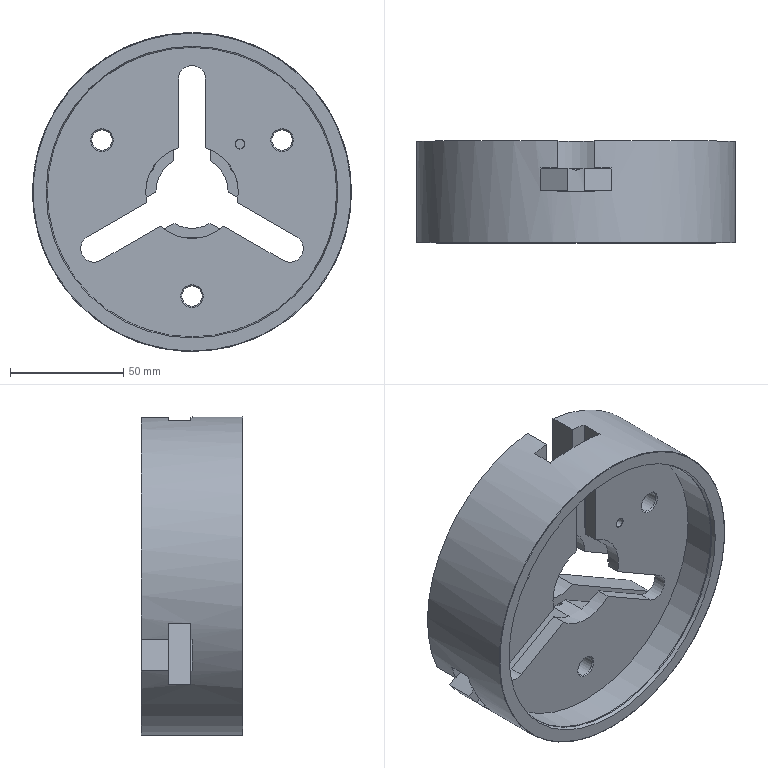CAM job | NX | 3-axis milling, drilling | part box 141 x 45 x 141 mm | stock box 141 x 45 x 141 mm
Tools:
number,name,description,diameter,corner_radius,flute_length,length,flutes
0,D30,Milling Tool-T Cutter,30.0,,9.0,50.0,4
0,D12,Milling Tool-5 Parameters,12.0,0.0,50.0,75.0,2
0,D14,Milling Tool-5 Parameters,14.0,0.0,50.0,75.0,2
0,D9,Milling Tool-5 Parameters,9.0,0.0,50.0,75.0,2
0,D4.2,Milling Tool-5 Parameters,4.2,0.0,50.0,75.0,2
0,D4,Milling Tool-5 Parameters,4.0,1.0,30.0,30.0,4
8,C20,Milling Tool-5 Parameters,20.0,0.0,15.0,50.0,1
Operations:
program,operation,operation_type,tool,method,geometry_group,spindle_rpm,surface_speed,feed_per_tooth,feed_cut,feed_plunge,cut_length_mm,path_length_mm,cut_time_min,machine_time_min
ZK,DRILLING,Operation,D4,METHOD,WORKPIECE,3000.0,37.0,0.0417,500.0,0.0,30.0,535.094,0.06,0.1105
ZK,PECK_DRILLING,Operation,D4.2,METHOD,WORKPIECE,1600.0,21.0,100.0,200.0,0.0,46.5,375.446,0.0001,0.033
ZK,PECK_DRILLING_1,Operation,D9,METHOD,WORKPIECE,1200.0,33.0,80.0,160.0,0.0,105.0,575.462,0.0005,0.0476
ZK,PECK_DRILLING_1_COPY,Operation,D14,METHOD,WORKPIECE,1200.0,33.0,80.0,100.0,0.0,34.5,434.462,0.0003,0.0403
D16-C,PLANAR_MILL,PlanarMilling,D14,METHOD,WORKPIECE,3600.0,158.0,0.5,3600.0,100.0,2032.8,2304.2,0.5647,0.5918
D16-C,PLANAR_MILL_COPY,PlanarMilling,D14,METHOD,WORKPIECE,3600.0,158.0,0.5,3600.0,100.0,2032.8,2304.2,0.5647,0.5918
D16-C,PLANAR_MILL_COPY_1,PlanarMilling,D14,METHOD,WORKPIECE,3600.0,158.0,0.5,3600.0,100.0,2032.8,2304.2,0.5647,0.5918
D12-CAO,PLANAR_MILL_1,PlanarMilling,D12,METHOD,WORKPIECE,0.0,0.0,0.0,250.0,100.0,53.0,311.0,0.212,0.2378
D12-CAO,PLANAR_MILL_1_COPY,PlanarMilling,D12,METHOD,WORKPIECE,0.0,0.0,0.0,250.0,100.0,53.0,311.0,0.212,0.2378
D12-CAO,PLANAR_MILL_1_COPY_1,PlanarMilling,D12,METHOD,WORKPIECE,0.0,0.0,0.0,250.0,100.0,53.0,311.0,0.212,0.2378
T-30CAO-CJG,PLANAR_MILL_2_COPY,PlanarMilling,D30,METHOD,WORKPIECE,0.0,0.0,0.0,250.0,100.0,386.8,628.6,1.547,1.571
T-30CAO-CJG,PLANAR_MILL_2_COPY_COPY,PlanarMilling,D30,METHOD,WORKPIECE,0.0,0.0,0.0,250.0,100.0,386.8,628.6,1.547,1.571
T-30CAO-CJG,PLANAR_MILL_2_COPY_COPY_1,PlanarMilling,D30,METHOD,WORKPIECE,0.0,0.0,0.0,250.0,100.0,386.8,628.6,1.547,1.571
T30-JING,PLANAR_MILL_2_COPY_COPY_2,PlanarMilling,D30,METHOD,WORKPIECE,0.0,0.0,0.0,250.0,100.0,388.0,630.0,1.552,1.576
T30-JING,PLANAR_MILL_2_COPY_COPY_2_COPY,PlanarMilling,D30,METHOD,WORKPIECE,0.0,0.0,0.0,250.0,100.0,388.0,630.0,1.552,1.576
T30-JING,PLANAR_MILL_2_COPY_COPY_2_COPY_1,PlanarMilling,D30,METHOD,WORKPIECE,0.0,0.0,0.0,250.0,100.0,388.0,630.0,1.552,1.576
D16CAO-JING,PLANAR_MILL_COPY_2,PlanarMilling,D14,METHOD,WORKPIECE,3600.0,158.0,0.5,3600.0,100.0,170.0,413.0,0.0472,0.0715
D16CAO-JING,PLANAR_MILL_COPY_2_COPY,PlanarMilling,D14,METHOD,WORKPIECE,3600.0,158.0,0.5,3600.0,100.0,170.0,413.0,0.0472,0.0715
D16CAO-JING,PLANAR_MILL_COPY_2_COPY_1,PlanarMilling,D14,METHOD,WORKPIECE,3600.0,158.0,0.5,3600.0,100.0,170.0,413.0,0.0472,0.0715
DAOJIAO,DRILLING_1,Operation,C20,METHOD,WORKPIECE,1300.0,49.0,0.2308,300.0,0.0,18.0,318.446,0.06,0.09
DAOJIAO,DRILLING_1_COPY,Operation,C20,METHOD,WORKPIECE,1300.0,49.0,0.2308,300.0,0.0,33.0,431.462,0.11,0.1498
DAOJIAO,PLANAR_MILL_2,PlanarMilling,C20,METHOD,WORKPIECE,5000.0,314.0,0.4,2000.0,100.0,484.927,688.927,0.2425,0.2629